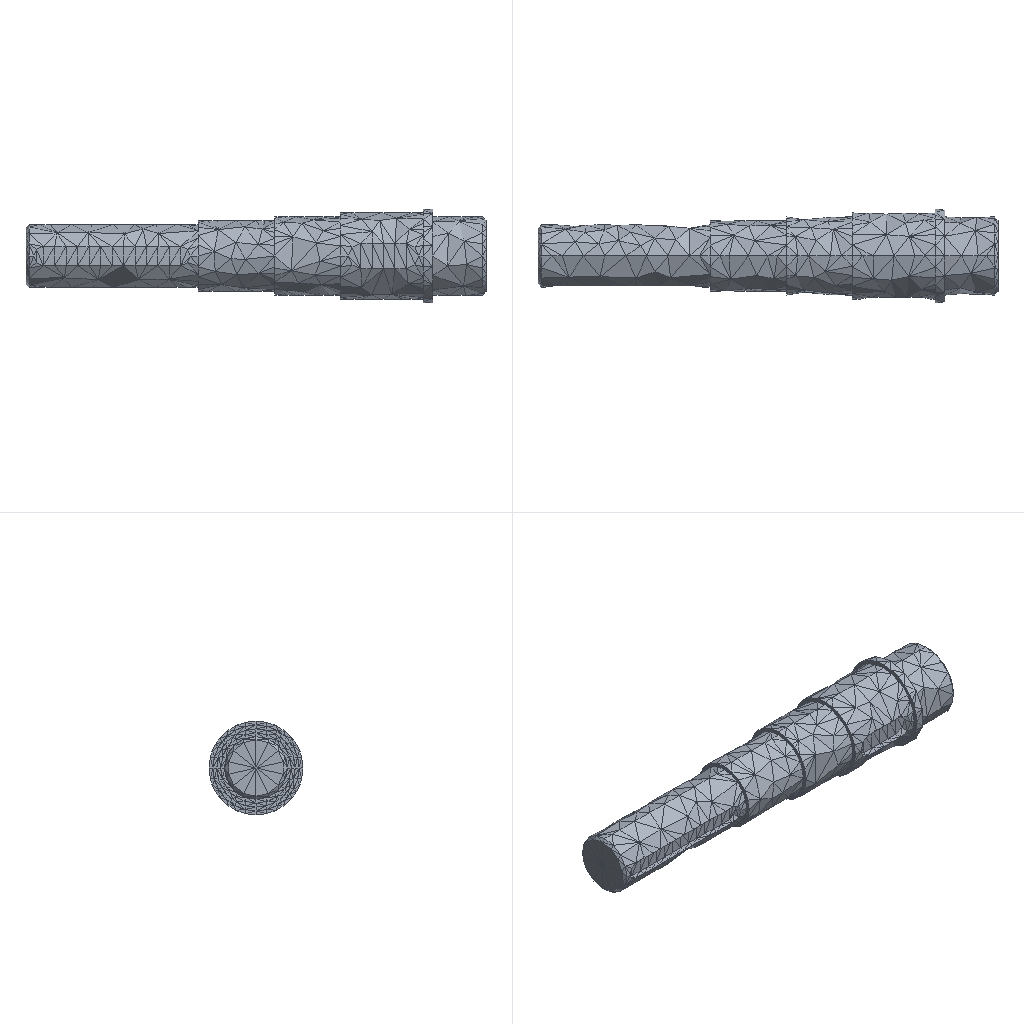Simulation study | ansys workbench
Set-up summary:
category,name,step,type,value,unit,region
solver,ansys_mapdl
solver,version,,,22.1
units,MPA,,stated
analysis,deck,,static,static
load_step,requested,,,1
analysis,nlgeom,,,False
mesh,nodes,,,4443
mesh,elements,,,2843
element_type,ANSYS 187 (type 1),,solid,2395
element_type,ANSYS 174 (type 2),,contact,448
element_type,ANSYS 170 (type 3),,target,0
load,load commands in deck,,count,3
bc,support commands in deck,,count,1
named_set,_FIXEDSU,,component
material,1,,in results
check,setup vs results,,match,results also hold 0 node(s) and 1 element(s) the deck makes with ['EN']; those were not compared; 1 node(s) the solver created internally for pilot nodes (ansys-fenxi-3/输出轴有限元分析报告/输出轴_files/dp0/SYS/MECH/solve.out) are in the results only
Ansys APDL input file, long lists of numbers shortened:
/batch
/config,noeldb,1     ! force off writing results to database
*get,_wallstrt,active,,time,wall
! ANSYS input file written by Workbench version 2022 R1
! File used for geometry attach: F:\ansys（分析文件汇总)\输出轴有限元分析报告\低速轴.STEP
/title,wbnew--____ (A5)
! ****** Begin Custom Load Command Snippet ******
/COM, ACT Extensions:
/COM,     LSDYNA, 2021.1
/COM,
! ****** End   Custom Load Command Snippet ******
*DIM,_wb_ProjectScratch_dir,string,248
_wb_ProjectScratch_dir(1) = 'C:\Users\Administrator\AppData\Local\Temp\WB_Administrator_332_2\_ProjectScratch\Scr0D24\'
*DIM,_wb_SolverFiles_dir,string,248
_wb_SolverFiles_dir(1) = 'C:\Users\Administrator\AppData\Local\Temp\WB_Administrator_332_2\wbnew_files\dp0\SYS\MECH\'
*DIM,_wb_userfiles_dir,string,248
_wb_userfiles_dir(1) = 'C:\Users\Administrator\AppData\Local\Temp\WB_Administrator_332_2\wbnew_files\user_files\'
/com,--- Data in consistent NMM units. See Solving Units in the help system for more information.
/units,MPA
/nopr
/wb,file,start              !  signify a WB generated input file
/prep7
! Turn off shape checking because checks already performed inside WB mesher.
! See help system for more information.
SHPP,OFF,,NOWARN
/nolist
etcon,set             ! allow ANSYS to choose best KEYOP's for 180x elements, resets any applicable keyopt to MAPDL defaults
/com,*********** Nodes for the whole assembly ***********
nblock,3,,4886
(1i9,3e20.9e3)
        1     0.000000000E+00     2.326828918E-15     1.800000000E+01
! (4441 more lines like these left out)
-1
/com,*********** Nodes for all Remote Points ***********
nblock,3
(1i9,3e20.9e3)
     4443     1.387784742E+02     1.502534316E+00    -4.770305994E-09
-1
/wb,elem,start            !  set before creation of elements
/com,*********** Elements for Body 1 "___-FreeParts|__2" ***********
et,1,187
eblock,19,solid,,2395
(19i9)
        1        1        1        1        0        0        0        0       10        0        1      589      736      666      733     3925     4343     3920     3924
! (4789 more lines like these left out)
-1
/wb,elem,end               !  done creating elements
/com,*********** Send User Defined Coordinate System(s) ***********
csys,0
toffst,273.15,  ! Temperature offset from absolute zero
/com,*********** Set Reference Temperature ***********
tref,22.
/wb,mat,start              !  starting to send materials
/com,*********** Send Materials ***********
Temperature = 'TEMP' ! Temperature
MP,DENS,1,7.85e-09,	! tonne mm^-3
MP,ALPX,1,1.2e-05,	! C^-1
MP,C,1,434000000,	! mm^2 s^-2 C^-1
MP,KXX,1,60.5,	! tonne mm s^-3 C^-1
MP,RSVX,1,0.00017,	! ohm mm
MP,EX,1,200000,	! tonne s^-2 mm^-1
MP,NUXY,1,0.3,
MP,MURX,1,10000,
/wb,mat,end                !  done sending materials
!************************* Model Summary ********************
!___-FreeParts|__2,	结构钢,	matid,	1
!************************* End Model Summary ********************
! get the diagonal of the bounding box. Needed later for other things
*get,_xmin,node,,mnloc,x
*get,_ymin,node,,mnloc,y
*get,_zmin,node,,mnloc,z
*get,_xmax,node,,mxloc,x
*get,_ymax,node,,mxloc,y
*get,_zmax,node,,mxloc,z
_ASMDIAG=(_xmax-_xmin)*(_xmax-_xmin)+(_ymax-_ymin)*(_ymax-_ymin)+(_zmax-_zmin)*(_zmax-_zmin)
_ASMDIAG=SQRT(_ASMDIAG)
/wb,contact,start          !  starting to send contact
/wb,contact,end            !  done creating contacts
/golist
/wb,load,start             !  starting to send loads
/com,*********** Fixed Supports ***********
CMBLOCK,_FIXEDSU,NODE,      448
(8i10)
        28        29        30        31        32        33        34        35
! (55 more lines like these left out)
cmsel,s,_FIXEDSU
d,all,all
nsel,all
/com,*********** Create Remote Point "内部远程点" ***********
! -------- Remote Point Used by "力矩" --------
*set,tid,3
*set,cid,2
et,cid,174
et,tid,170
keyo,tid,2,1               ! Don't fix the pilot node
keyo,tid,4,111111
keyo,cid,12,5              ! Bonded Contact
keyo,cid,4,1               ! Deformable RBE3 style load
keyo,cid,2,2               ! MPC style contact
eblock,10,,,448
(15i9)
     3549        2        2        2        0      298      436      550      550     2645     3167      550     2646
! (447 more lines like these left out)
-1
*set,_npilot,4443
_npilot30=_npilot
type,tid
mat ,cid
real,cid
tshape,pilo
en,3997,_npilot
tshape
/com,*********** Construct Moment Using Remote Attachment ***********
/gst,on,on
fini
*get,_numnode,node,0,count
*get,_numelem,elem,0,count
*get, _MAXELEMNUM, elem, 0, NUM, MAX
*get, _MAXNODENUM, node, 0, NUM, MAX
*get, _MAXELEMTYPE, etyp, 0, NUM, MAX
*get, _MAXREALCONST, real, 0, NUM, MAX
/go
/wb,load,end               !  done creating loads
/com,--- Number of total nodes = %_numnode%
/com,--- Number of contact elements = 448
/com,--- Number of spring elements = 0
/com,--- Number of bearing elements = 0
/com,--- Number of solid elements = 2395
/com,--- Number of condensed parts = 0
/com,--- Number of total elements = %_numelem%
*get,_wallbsol,active,,time,wall
/com,****************************************************************************
/com,*************************    SOLUTION       ********************************
/com,****************************************************************************
/solu
antype,0                   ! static analysis
_thickRatio=  1     ! Ratio of thick parts in the model
eqsl,pcg,1e-8,,,,,,1
cntr,print,1               ! print out contact info and also make no initial contact an error
dmpoption,emat,no             ! Don't combine emat file for DANSYS
dmpoption,esav,no             ! Don't combine esav file for DANSYS
nldiag,cont,iter           ! print out contact info each equilibrium iteration
rescontrol,,none                 ! Do not keep any restart files
/com,****************************************************
/com,******************* SOLVE FOR LS 1 OF 1 ****************
nsel,s,node,,4443
f,all,mx,500.
f,all,my,0.
f,all,mz,0.
nsel,all
/nopr
/gopr
nsub,1,1,1
time,1.
outres,erase
outres,all,none
outres,nsol,all,
outres,rsol,all
outres,eangl,all
outres,etmp,all
outres,veng,all
outres,strs,all,
outres,epel,all,
outres,eppl,all,
outres,cont,all,
! *********** WB SOLVE COMMAND ***********
! check interactive state
*get,ANSINTER_,active,,int
*if,ANSINTER_,ne,0,then
/eof
*endif
solve
/com *************** Write FE CONNECTORS *********
CEWRITE,file,ce,,INTE
/com,****************************************************
/com,*************** FINISHED SOLVE FOR LS 1 *************
*get,_wallasol,active,,time,wall
/nopr
*get,_numnode,node,0,count
*get,_numelem,elem,0,count
*get, _MAXELEMNUM, elem, 0, NUM, MAX
*get, _MAXNODENUM, node, 0, NUM, MAX,,,INTERNAL
*get, _MAXELEMTYPE, etyp, 0, NUM, MAX
*get, _MAXREALCONST, real, 0, NUM, MAX
/gopr
*get,_PCGITER,active,,solu,cgiter
/post1
xmlo,ENCODING,ISO-8859-1
xmlo,parm
/xml,parm,xml
fini
/gopr
*get,_walldone,active,,time,wall
_preptime=(_wallbsol-_wallstrt)*3600
_solvtime=(_wallasol-_wallbsol)*3600
_posttime=(_walldone-_wallasol)*3600
_totaltim=(_walldone-_wallstrt)*3600
*get,_dlbratio,active,0,solu,dlbr
*get,_combtime,active,0,solu,comb
*get,_ssmode,active,0,solu,ssmm
*get,_ndofs,active,0,solu,ndof
*get,_sol_end_time,active,0,set,time
*if,_sol_end_time,eq,1.,then
/fclean				!clean distributed files
*endif
/com,--- Total number of nodes = %_numnode%
/com,--- Total number of elements = %_numelem%
/com,--- Element load balance ratio = %_dlbratio%
/com,--- Time to combine distributed files = %_combtime%
/com,--- Sparse memory mode = %_ssmode%
/com,--- Number of DOF = %_ndofs%
/wb,file,end               ! done with WB generated input
Results summary:
result,analysis,,,static
result,last_loadstep,,,1
result,primary field,,,displacement
result,reaction total,1,FX,-0.0,N
result,reaction total,1,FY,0.0,N
result,reaction total,1,FZ,0.0,N
result,mass,,,0.003916,"NMM: mm, ton, N, s, mV, mA, degC"